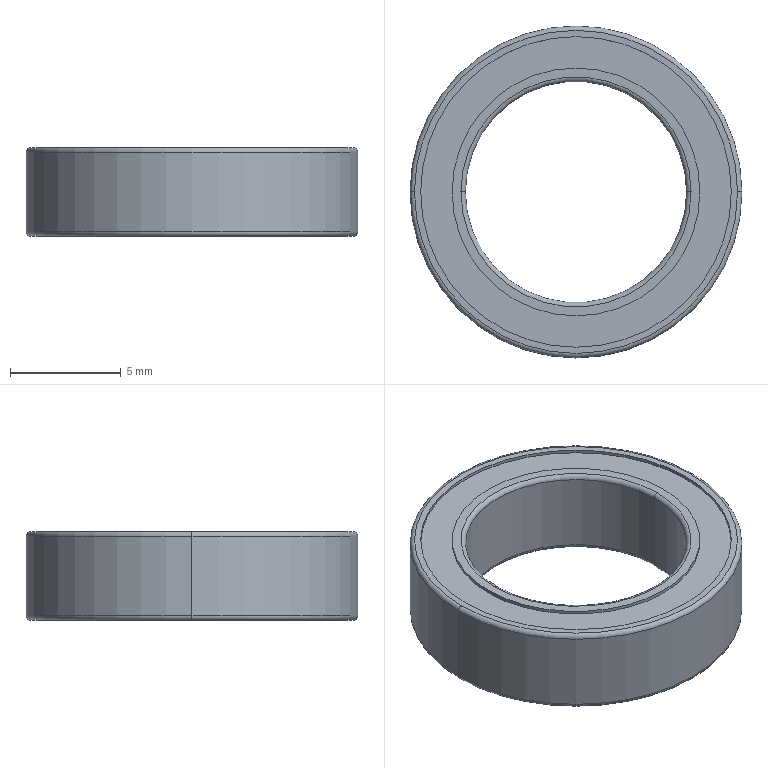Part | STEP file | B6700ZZ_C-B6700ZZ | 1 solid | 26 faces | box 15 x 15 x 4 mm | volume 375.474 mm3 | cylinder 12 | torus 8 | plane 6 | commonest cylinder face diameters 11.2 x4 14.04 x4 10 x2 15 x2